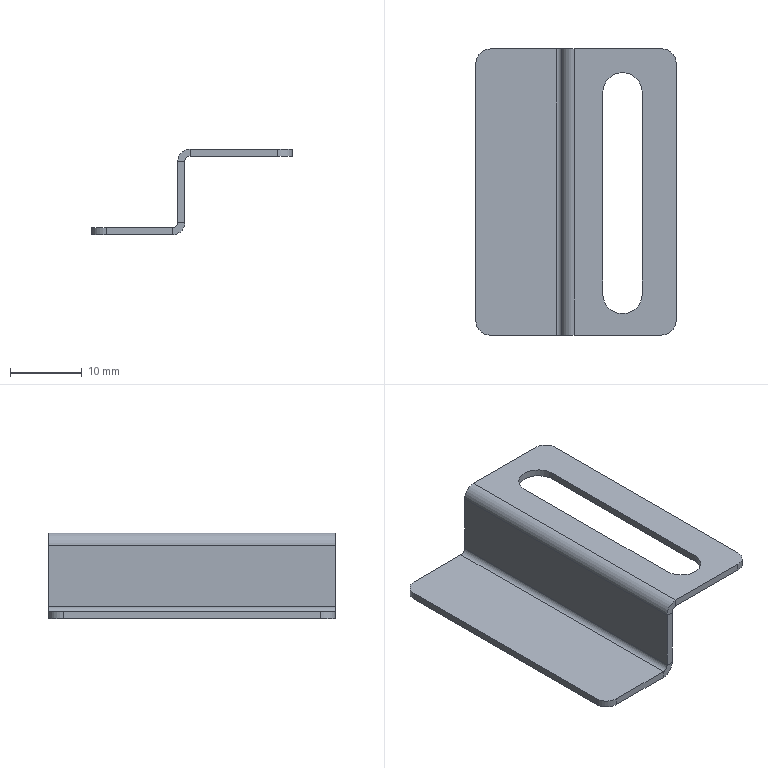Part | STEP file | ND25021-08-JDKM-03-BJ | 1 solid | 30 faces | box 28 x 40 x 12 mm | volume 1335 mm3 | plane 20 | cylinder 10 | commonest cylinder face diameters 4 x4 1.473 x2 3.473 x2 5.5 x2